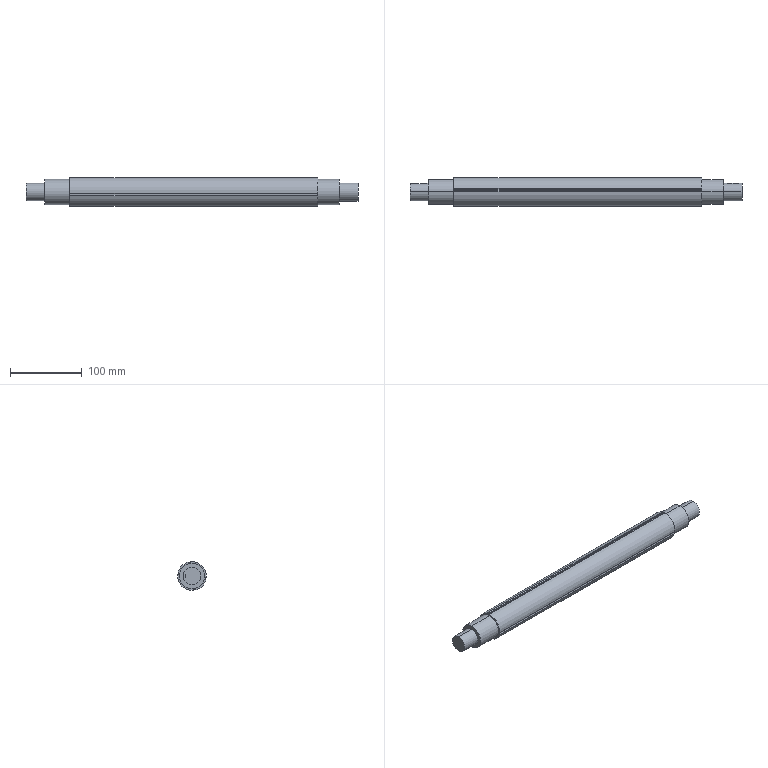Part | SolidWorks | features ICE 7, RefAxis 3, 3DProfileFeature 1, LockFeature 1, MirrorPattern 1, MoveFace 1, Revolution 1 | 1 solid | 34 faces | box 462 x 40 x 40 mm | volume 516055 mm3 | cylinder 22 | plane 12 | commonest cylinder face diameters 4.38 x5 40 x5 8 x4 35 x4 24 x2 25 x2
STEP:
#1=CARTESIAN_POINT('',(185.5,11.843,-4.));
#2=VERTEX_POINT('',#1);
#3=CARTESIAN_POINT('',(185.5,11.843,4.));
#4=VERTEX_POINT('',#3);
#5=CARTESIAN_POINT('',(185.5,11.843,-4.));
#6=CARTESIAN_POINT('',(185.234,11.843,-4.));
#7=CARTESIAN_POINT('',(184.973,11.852,-3.974));
#8=CARTESIAN_POINT('',(184.459,11.886,-3.871));
#9=CARTESIAN_POINT('',(184.204,11.911,-3.793));
#10=CARTESIAN_POINT('',(183.721,11.973,-3.592));
#11=CARTESIAN_POINT('',(183.492,12.01,-3.469));
#12=CARTESIAN_POINT('',(183.059,12.09,-3.179));
#13=CARTESIAN_POINT('',(182.855,12.133,-3.012));
#14=CARTESIAN_POINT('',(182.489,12.218,-2.646));
#15=CARTESIAN_POINT('',(182.324,12.26,-2.445));
#16=CARTESIAN_POINT('',(182.031,12.34,-2.009));
#17=CARTESIAN_POINT('',(181.908,12.375,-1.779));
#18=CARTESIAN_POINT('',(181.708,12.435,-1.299));
#19=CARTESIAN_POINT('',(181.63,12.459,-1.045));
#20=CARTESIAN_POINT('',(181.526,12.492,-0.5276));
#21=CARTESIAN_POINT('',(181.5,12.5,-0.2669));
#22=CARTESIAN_POINT('',(181.5,12.5,0.2587));
#23=CARTESIAN_POINT('',(181.526,12.492,0.5256));
#24=CARTESIAN_POINT('',(181.629,12.459,1.04));
#25=CARTESIAN_POINT('',(181.705,12.436,1.29));
#26=CARTESIAN_POINT('',(181.907,12.375,1.777));
#27=CARTESIAN_POINT('',(182.031,12.34,2.008));
#28=CARTESIAN_POINT('',(182.32,12.262,2.44));
#29=CARTESIAN_POINT('',(182.487,12.219,2.643));
#30=CARTESIAN_POINT('',(182.855,12.133,3.012));
#31=CARTESIAN_POINT('',(183.055,12.091,3.176));
#32=CARTESIAN_POINT('',(183.487,12.011,3.466));
#33=CARTESIAN_POINT('',(183.72,11.973,3.592));
#34=CARTESIAN_POINT('',(184.202,11.911,3.792));
#35=CARTESIAN_POINT('',(184.451,11.886,3.869));
#36=CARTESIAN_POINT('',(184.968,11.852,3.973));
#37=CARTESIAN_POINT('',(185.234,11.843,4.));
#38=CARTESIAN_POINT('',(185.5,11.843,4.));
#39=B_SPLINE_CURVE_WITH_KNOTS('',3,(#5,#6,#7,#8,#9,#10,#11,#12,#13,#14,#15,#16,#17,#18,#19,#20,#21,#22,#23,#24,#25,#26,#27,#28,#29,#30,#31,#32,#33,#34,#35,#36,#37,#38),.UNSPECIFIED.,.F.,.F.,(4,2,2,2,2,2,2,2,2,2,2,2,2,2,2,2,4),(0.,0.0007865,0.001573,0.00236,0.003146,0.003933,0.004719,0.005506,0.006292,0.007079,0.007865,0.008652,0.009438,0.01022,0.01101,0.0118,0.01258),.UNSPECIFIED.);
#40=EDGE_CURVE('',#2,#4,#39,.T.);
#41=ORIENTED_EDGE('',*,*,#40,.F.);
#42=CARTESIAN_POINT('',(200.5,11.843,-4.));
#43=VERTEX_POINT('',#42);
#44=CARTESIAN_POINT('',(179.5,11.843,-4.));
#45=DIRECTION('',(-1.,0.,0.));
#46=VECTOR('',#45,1000.);
#47=LINE('',#44,#46);
#48=EDGE_CURVE('',#43,#2,#47,.T.);
#49=ORIENTED_EDGE('',*,*,#48,.F.);
#50=CARTESIAN_POINT('',(200.5,11.843,4.));
#51=VERTEX_POINT('',#50);
#52=CARTESIAN_POINT('',(200.5,11.843,4.));
#53=CARTESIAN_POINT('',(200.766,11.843,4.));
#54=CARTESIAN_POINT('',(201.027,11.852,3.974));
#55=CARTESIAN_POINT('',(201.541,11.886,3.871));
#56=CARTESIAN_POINT('',(201.796,11.911,3.793));
#57=CARTESIAN_POINT('',(202.279,11.973,3.592));
#58=CARTESIAN_POINT('',(202.508,12.01,3.469));
#59=CARTESIAN_POINT('',(202.941,12.09,3.179));
#60=CARTESIAN_POINT('',(203.145,12.133,3.012));
#61=CARTESIAN_POINT('',(203.511,12.218,2.646));
#62=CARTESIAN_POINT('',(203.676,12.26,2.445));
#63=CARTESIAN_POINT('',(203.969,12.34,2.009));
#64=CARTESIAN_POINT('',(204.092,12.375,1.779));
#65=CARTESIAN_POINT('',(204.292,12.435,1.299));
#66=CARTESIAN_POINT('',(204.37,12.459,1.045));
#67=CARTESIAN_POINT('',(204.474,12.492,0.5276));
#68=CARTESIAN_POINT('',(204.5,12.5,0.2669));
#69=CARTESIAN_POINT('',(204.5,12.5,-0.2587));
#70=CARTESIAN_POINT('',(204.474,12.492,-0.5256));
#71=CARTESIAN_POINT('',(204.371,12.459,-1.04));
#72=CARTESIAN_POINT('',(204.295,12.436,-1.29));
#73=CARTESIAN_POINT('',(204.093,12.375,-1.777));
#74=CARTESIAN_POINT('',(203.969,12.34,-2.008));
#75=CARTESIAN_POINT('',(203.68,12.262,-2.44));
#76=CARTESIAN_POINT('',(203.513,12.219,-2.643));
#77=CARTESIAN_POINT('',(203.145,12.133,-3.012));
#78=CARTESIAN_POINT('',(202.945,12.091,-3.176));
#79=CARTESIAN_POINT('',(202.513,12.011,-3.466));
#80=CARTESIAN_POINT('',(202.28,11.973,-3.592));
#81=CARTESIAN_POINT('',(201.798,11.911,-3.792));
#82=CARTESIAN_POINT('',(201.549,11.886,-3.869));
#83=CARTESIAN_POINT('',(201.032,11.852,-3.973));
#84=CARTESIAN_POINT('',(200.766,11.843,-4.));
#85=CARTESIAN_POINT('',(200.5,11.843,-4.));
#86=B_SPLINE_CURVE_WITH_KNOTS('',3,(#52,#53,#54,#55,#56,#57,#58,#59,#60,#61,#62,#63,#64,#65,#66,#67,#68,#69,#70,#71,#72,#73,#74,#75,#76,#77,#78,#79,#80,#81,#82,#83,#84,#85),.UNSPECIFIED.,.F.,.F.,(4,2,2,2,2,2,2,2,2,2,2,2,2,2,2,2,4),(0.,0.0007865,0.001573,0.00236,0.003146,0.003933,0.004719,0.005506,0.006292,0.007079,0.007865,0.008652,0.009438,0.01022,0.01101,0.0118,0.01258),.UNSPECIFIED.);
#87=EDGE_CURVE('',#51,#43,#86,.T.);
#88=ORIENTED_EDGE('',*,*,#87,.F.);
#89=CARTESIAN_POINT('',(179.5,11.843,4.));
#90=DIRECTION('',(1.,0.,0.));
#91=VECTOR('',#90,1000.);
#92=LINE('',#89,#91);
#93=EDGE_CURVE('',#4,#51,#92,.T.);
#94=ORIENTED_EDGE('',*,*,#93,.F.);
#95=EDGE_LOOP('',(#41,#49,#88,#94));
#96=FACE_BOUND('',#95,.T.);
#97=CARTESIAN_POINT('',(179.5,0.,-12.5));
#98=VERTEX_POINT('',#97);
#99=CARTESIAN_POINT('',(179.5,0.,12.5));
#100=VERTEX_POINT('',#99);
#101=CARTESIAN_POINT('',(179.5,0.,0.));
#102=DIRECTION('',(1.,0.,0.));
#103=DIRECTION('',(0.,0.,-1.));
#104=AXIS2_PLACEMENT_3D('',#101,#102,#103);
#105=CIRCLE('',#104,12.5);
#106=EDGE_CURVE('',#98,#100,#105,.T.);
#107=ORIENTED_EDGE('',*,*,#106,.T.);
#108=CARTESIAN_POINT('',(205.5,0.,12.5));
#109=VERTEX_POINT('',#108);
#110=CARTESIAN_POINT('',(179.5,0.,12.5));
#111=DIRECTION('',(1.,0.,0.));
#112=VECTOR('',#111,1000.);
#113=LINE('',#110,#112);
#114=EDGE_CURVE('',#100,#109,#113,.T.);
#115=ORIENTED_EDGE('',*,*,#114,.T.);
#116=CARTESIAN_POINT('',(205.5,0.,-12.5));
#117=VERTEX_POINT('',#116);
#118=CARTESIAN_POINT('',(205.5,0.,0.));
#119=DIRECTION('',(1.,0.,0.));
#120=DIRECTION('',(0.,0.,-1.));
#121=AXIS2_PLACEMENT_3D('',#118,#119,#120);
#122=CIRCLE('',#121,12.5);
#123=EDGE_CURVE('',#117,#109,#122,.T.);
#124=ORIENTED_EDGE('',*,*,#123,.F.);
#125=CARTESIAN_POINT('',(179.5,0.,-12.5));
#126=DIRECTION('',(1.,0.,0.));
#127=VECTOR('',#126,1000.);
#128=LINE('',#125,#127);
#129=EDGE_CURVE('',#98,#117,#128,.T.);
#130=ORIENTED_EDGE('',*,*,#129,.F.);
#131=EDGE_LOOP('',(#107,#115,#124,#130));
#132=FACE_OUTER_BOUND('',#131,.T.);
#133=CARTESIAN_POINT('',(179.5,0.,0.));
#134=DIRECTION('',(1.,0.,0.));
#135=DIRECTION('',(0.,0.,-1.));
#136=AXIS2_PLACEMENT_3D('',#133,#134,#135);
#137=CYLINDRICAL_SURFACE('',#136,12.5);
#138=ADVANCED_FACE('',(#96,#132),#137,.T.);
#139=CARTESIAN_POINT('',(149.5,0.,-17.5));
#140=VERTEX_POINT('',#139);
#141=CARTESIAN_POINT('',(149.5,0.,17.5));
#142=VERTEX_POINT('',#141);
#143=CARTESIAN_POINT('',(149.5,0.,0.));
#144=DIRECTION('',(1.,0.,0.));
#145=DIRECTION('',(0.,0.,-1.));
#146=AXIS2_PLACEMENT_3D('',#143,#144,#145);
#147=CIRCLE('',#146,17.5);
#148=EDGE_CURVE('',#140,#142,#147,.T.);
#149=ORIENTED_EDGE('',*,*,#148,.T.);
#150=CARTESIAN_POINT('',(179.5,0.,17.5));
#151=VERTEX_POINT('',#150);
#152=CARTESIAN_POINT('',(149.5,0.,17.5));
#153=DIRECTION('',(1.,0.,0.));
#154=VECTOR('',#153,1000.);
#155=LINE('',#152,#154);
#156=EDGE_CURVE('',#142,#151,#155,.T.);
#157=ORIENTED_EDGE('',*,*,#156,.T.);
#158=CARTESIAN_POINT('',(179.5,0.,-17.5));
#159=VERTEX_POINT('',#158);
#160=CARTESIAN_POINT('',(179.5,0.,0.));
#161=DIRECTION('',(1.,0.,0.));
#162=DIRECTION('',(0.,0.,-1.));
#163=AXIS2_PLACEMENT_3D('',#160,#161,#162);
#164=CIRCLE('',#163,17.5);
#165=EDGE_CURVE('',#159,#151,#164,.T.);
#166=ORIENTED_EDGE('',*,*,#165,.F.);
#167=CARTESIAN_POINT('',(149.5,0.,-17.5));
#168=DIRECTION('',(1.,0.,0.));
#169=VECTOR('',#168,1000.);
#170=LINE('',#167,#169);
#171=EDGE_CURVE('',#140,#159,#170,.T.);
#172=ORIENTED_EDGE('',*,*,#171,.F.);
#173=EDGE_LOOP('',(#149,#157,#166,#172));
#174=FACE_OUTER_BOUND('',#173,.T.);
#175=CARTESIAN_POINT('',(149.5,0.,0.));
#176=DIRECTION('',(1.,0.,0.));
#177=DIRECTION('',(0.,0.,-1.));
#178=AXIS2_PLACEMENT_3D('',#175,#176,#177);
#179=CYLINDRICAL_SURFACE('',#178,17.5);
#180=ADVANCED_FACE('',(#174),#179,.T.);
#181=CARTESIAN_POINT('',(-195.5,5.203,19.311));
#182=VERTEX_POINT('',#181);
#183=CARTESIAN_POINT('',(-195.5,3.683,18.698));
#184=VERTEX_POINT('',#183);
#185=CARTESIAN_POINT('',(-195.5,3.683,20.888));
#186=DIRECTION('',(-1.,0.,0.));
#187=DIRECTION('',(0.,0.,1.));
#188=AXIS2_PLACEMENT_3D('',#185,#186,#187);
#189=CIRCLE('',#188,2.19);
#190=EDGE_CURVE('',#182,#184,#189,.T.);
#191=ORIENTED_EDGE('',*,*,#190,.T.);
#192=CARTESIAN_POINT('',(149.5,3.683,18.698));
#193=VERTEX_POINT('',#192);
#194=CARTESIAN_POINT('',(-205.5,3.683,18.698));
#195=DIRECTION('',(1.,0.,0.));
#196=VECTOR('',#195,1000.);
#197=LINE('',#194,#196);
#198=EDGE_CURVE('',#184,#193,#197,.T.);
#199=ORIENTED_EDGE('',*,*,#198,.T.);
#200=CARTESIAN_POINT('',(149.5,5.203,19.311));
#201=VERTEX_POINT('',#200);
#202=CARTESIAN_POINT('',(149.5,3.683,20.888));
#203=DIRECTION('',(1.,0.,0.));
#204=DIRECTION('',(0.,0.,-1.));
#205=AXIS2_PLACEMENT_3D('',#202,#203,#204);
#206=CIRCLE('',#205,2.19);
#207=EDGE_CURVE('',#193,#201,#206,.T.);
#208=ORIENTED_EDGE('',*,*,#207,.T.);
#209=CARTESIAN_POINT('',(-205.5,5.203,19.311));
#210=DIRECTION('',(1.,0.,0.));
#211=VECTOR('',#210,1000.);
#212=LINE('',#209,#211);
#213=EDGE_CURVE('',#182,#201,#212,.T.);
#214=ORIENTED_EDGE('',*,*,#213,.F.);
#215=EDGE_LOOP('',(#191,#199,#208,#214));
#216=FACE_OUTER_BOUND('',#215,.T.);
#217=CARTESIAN_POINT('',(-205.5,3.683,20.888));
#218=DIRECTION('',(1.,0.,0.));
#219=DIRECTION('',(0.,0.,-1.));
#220=AXIS2_PLACEMENT_3D('',#217,#218,#219);
#221=CYLINDRICAL_SURFACE('',#220,2.19);
#222=ADVANCED_FACE('',(#216),#221,.F.);
#223=CARTESIAN_POINT('',(149.5,0.,20.));
#224=VERTEX_POINT('',#223);
#225=CARTESIAN_POINT('',(149.5,-19.926,-1.715));
#226=VERTEX_POINT('',#225);
#227=CARTESIAN_POINT('',(149.5,0.,0.));
#228=DIRECTION('',(1.,0.,0.));
#229=DIRECTION('',(0.,0.,-1.));
#230=AXIS2_PLACEMENT_3D('',#227,#228,#229);
#231=CIRCLE('',#230,20.);
#232=EDGE_CURVE('',#224,#226,#231,.T.);
#233=ORIENTED_EDGE('',*,*,#232,.F.);
#234=CARTESIAN_POINT('',(-195.5,0.,20.));
#235=VERTEX_POINT('',#234);
#236=CARTESIAN_POINT('',(205.5,0.,20.));
#237=DIRECTION('',(-1.,0.,0.));
#238=VECTOR('',#237,1000.);
#239=LINE('',#236,#238);
#240=EDGE_CURVE('',#224,#235,#239,.T.);
#241=ORIENTED_EDGE('',*,*,#240,.T.);
#242=CARTESIAN_POINT('',(-195.5,-19.926,-1.715));
#243=VERTEX_POINT('',#242);
#244=CARTESIAN_POINT('',(-195.5,0.,0.));
#245=DIRECTION('',(-1.,0.,0.));
#246=DIRECTION('',(0.,0.,1.));
#247=AXIS2_PLACEMENT_3D('',#244,#245,#246);
#248=CIRCLE('',#247,20.);
#249=EDGE_CURVE('',#243,#235,#248,.T.);
#250=ORIENTED_EDGE('',*,*,#249,.F.);
#251=CARTESIAN_POINT('',(-205.5,-19.926,-1.715));
#252=DIRECTION('',(1.,0.,0.));
#253=VECTOR('',#252,1000.);
#254=LINE('',#251,#253);
#255=EDGE_CURVE('',#243,#226,#254,.T.);
#256=ORIENTED_EDGE('',*,*,#255,.T.);
#257=EDGE_LOOP('',(#233,#241,#250,#256));
#258=FACE_OUTER_BOUND('',#257,.T.);
#259=CARTESIAN_POINT('',(205.5,0.,0.));
#260=DIRECTION('',(-1.,0.,0.));
#261=DIRECTION('',(0.,0.,1.));
#262=AXIS2_PLACEMENT_3D('',#259,#260,#261);
#263=CYLINDRICAL_SURFACE('',#262,20.);
#264=ADVANCED_FACE('',(#258),#263,.T.);
#265=CARTESIAN_POINT('',(-195.5,0.,17.5));
#266=VERTEX_POINT('',#265);
#267=CARTESIAN_POINT('',(-195.5,0.,-17.5));
#268=VERTEX_POINT('',#267);
#269=CARTESIAN_POINT('',(-195.5,0.,0.));
#270=DIRECTION('',(-1.,0.,0.));
#271=DIRECTION('',(0.,0.,1.));
#272=AXIS2_PLACEMENT_3D('',#269,#270,#271);
#273=CIRCLE('',#272,17.5);
#274=EDGE_CURVE('',#266,#268,#273,.T.);
#275=ORIENTED_EDGE('',*,*,#274,.T.);
#276=CARTESIAN_POINT('',(-230.5,0.,-17.5));
#277=VERTEX_POINT('',#276);
#278=CARTESIAN_POINT('',(-187.5,0.,-17.5));
#279=DIRECTION('',(-1.,0.,0.));
#280=VECTOR('',#279,1000.);
#281=LINE('',#278,#280);
#282=EDGE_CURVE('',#268,#277,#281,.T.);
#283=ORIENTED_EDGE('',*,*,#282,.T.);
#284=CARTESIAN_POINT('',(-230.5,0.,17.5));
#285=VERTEX_POINT('',#284);
#286=CARTESIAN_POINT('',(-230.5,0.,0.));
#287=DIRECTION('',(1.,0.,0.));
#288=DIRECTION('',(0.,0.,1.));
#289=AXIS2_PLACEMENT_3D('',#286,#287,#288);
#290=CIRCLE('',#289,17.5);
#291=EDGE_CURVE('',#277,#285,#290,.T.);
#292=ORIENTED_EDGE('',*,*,#291,.T.);
#293=CARTESIAN_POINT('',(-187.5,0.,17.5));
#294=DIRECTION('',(-1.,0.,0.));
#295=VECTOR('',#294,1000.);
#296=LINE('',#293,#295);
#297=EDGE_CURVE('',#266,#285,#296,.T.);
#298=ORIENTED_EDGE('',*,*,#297,.F.);
#299=EDGE_LOOP('',(#275,#283,#292,#298));
#300=FACE_OUTER_BOUND('',#299,.T.);
#301=CARTESIAN_POINT('',(-187.5,0.,0.));
#302=DIRECTION('',(-1.,0.,0.));
#303=DIRECTION('',(0.,0.,1.));
#304=AXIS2_PLACEMENT_3D('',#301,#302,#303);
#305=CYLINDRICAL_SURFACE('',#304,17.5);
#306=ADVANCED_FACE('',(#300),#305,.T.);
#307=CARTESIAN_POINT('',(-236.5,11.314,4.));
#308=VERTEX_POINT('',#307);
#309=CARTESIAN_POINT('',(-251.5,11.314,4.));
#310=VERTEX_POINT('',#309);
#311=CARTESIAN_POINT('',(-230.5,11.314,4.));
#312=DIRECTION('',(-1.,0.,0.));
#313=VECTOR('',#312,1000.);
#314=LINE('',#311,#313);
#315=EDGE_CURVE('',#308,#310,#314,.T.);
#316=ORIENTED_EDGE('',*,*,#315,.T.);
#317=CARTESIAN_POINT('',(-251.5,11.314,-4.));
#318=VERTEX_POINT('',#317);
#319=CARTESIAN_POINT('',(-251.5,11.314,4.));
#320=CARTESIAN_POINT('',(-251.766,11.314,4.));
#321=CARTESIAN_POINT('',(-252.028,11.323,3.974));
#322=CARTESIAN_POINT('',(-252.541,11.359,3.871));
#323=CARTESIAN_POINT('',(-252.796,11.385,3.793));
#324=CARTESIAN_POINT('',(-253.279,11.45,3.592));
#325=CARTESIAN_POINT('',(-253.508,11.489,3.469));
#326=CARTESIAN_POINT('',(-253.942,11.572,3.179));
#327=CARTESIAN_POINT('',(-254.145,11.617,3.012));
#328=CARTESIAN_POINT('',(-254.511,11.706,2.646));
#329=CARTESIAN_POINT('',(-254.676,11.75,2.446));
#330=CARTESIAN_POINT('',(-254.969,11.833,2.009));
#331=CARTESIAN_POINT('',(-255.092,11.87,1.78));
#332=CARTESIAN_POINT('',(-255.292,11.932,1.299));
#333=CARTESIAN_POINT('',(-255.37,11.957,1.045));
#334=CARTESIAN_POINT('',(-255.474,11.991,0.528));
#335=CARTESIAN_POINT('',(-255.5,12.,0.2672));
#336=CARTESIAN_POINT('',(-255.5,12.,-0.2587));
#337=CARTESIAN_POINT('',(-255.474,11.991,-0.5259));
#338=CARTESIAN_POINT('',(-255.371,11.958,-1.04));
#339=CARTESIAN_POINT('',(-255.295,11.933,-1.291));
#340=CARTESIAN_POINT('',(-255.093,11.87,-1.778));
#341=CARTESIAN_POINT('',(-254.969,11.833,-2.009));
#342=CARTESIAN_POINT('',(-254.68,11.751,-2.44));
#343=CARTESIAN_POINT('',(-254.513,11.707,-2.644));
#344=CARTESIAN_POINT('',(-254.145,11.617,-3.012));
#345=CARTESIAN_POINT('',(-253.945,11.573,-3.176));
#346=CARTESIAN_POINT('',(-253.514,11.49,-3.466));
#347=CARTESIAN_POINT('',(-253.28,11.45,-3.592));
#348=CARTESIAN_POINT('',(-252.799,11.386,-3.792));
#349=CARTESIAN_POINT('',(-252.55,11.359,-3.869));
#350=CARTESIAN_POINT('',(-252.032,11.323,-3.973));
#351=CARTESIAN_POINT('',(-251.766,11.314,-4.));
#352=CARTESIAN_POINT('',(-251.5,11.314,-4.));
#353=B_SPLINE_CURVE_WITH_KNOTS('',3,(#319,#320,#321,#322,#323,#324,#325,#326,#327,#328,#329,#330,#331,#332,#333,#334,#335,#336,#337,#338,#339,#340,#341,#342,#343,#344,#345,#346,#347,#348,#349,#350,#351,#352),.UNSPECIFIED.,.F.,.F.,(4,2,2,2,2,2,2,2,2,2,2,2,2,2,2,2,4),(0.,0.000787,0.001574,0.002361,0.003148,0.003935,0.004722,0.005509,0.006296,0.007083,0.00787,0.008657,0.009444,0.01023,0.01102,0.0118,0.01259),.UNSPECIFIED.);
#354=EDGE_CURVE('',#310,#318,#353,.T.);
#355=ORIENTED_EDGE('',*,*,#354,.T.);
#356=CARTESIAN_POINT('',(-236.5,11.314,-4.));
#357=VERTEX_POINT('',#356);
#358=CARTESIAN_POINT('',(-230.5,11.314,-4.));
#359=DIRECTION('',(1.,0.,0.));
#360=VECTOR('',#359,1000.);
#361=LINE('',#358,#360);
#362=EDGE_CURVE('',#318,#357,#361,.T.);
#363=ORIENTED_EDGE('',*,*,#362,.T.);
#364=CARTESIAN_POINT('',(-236.5,11.314,-4.));
#365=CARTESIAN_POINT('',(-236.234,11.314,-4.));
#366=CARTESIAN_POINT('',(-235.972,11.323,-3.974));
#367=CARTESIAN_POINT('',(-235.459,11.359,-3.871));
#368=CARTESIAN_POINT('',(-235.204,11.385,-3.793));
#369=CARTESIAN_POINT('',(-234.721,11.45,-3.592));
#370=CARTESIAN_POINT('',(-234.492,11.489,-3.469));
#371=CARTESIAN_POINT('',(-234.058,11.572,-3.179));
#372=CARTESIAN_POINT('',(-233.855,11.617,-3.012));
#373=CARTESIAN_POINT('',(-233.489,11.706,-2.646));
#374=CARTESIAN_POINT('',(-233.324,11.75,-2.446));
#375=CARTESIAN_POINT('',(-233.031,11.833,-2.009));
#376=CARTESIAN_POINT('',(-232.908,11.87,-1.78));
#377=CARTESIAN_POINT('',(-232.708,11.932,-1.299));
#378=CARTESIAN_POINT('',(-232.63,11.957,-1.045));
#379=CARTESIAN_POINT('',(-232.526,11.991,-0.528));
#380=CARTESIAN_POINT('',(-232.5,12.,-0.2672));
#381=CARTESIAN_POINT('',(-232.5,12.,0.2587));
#382=CARTESIAN_POINT('',(-232.526,11.991,0.5259));
#383=CARTESIAN_POINT('',(-232.629,11.958,1.04));
#384=CARTESIAN_POINT('',(-232.705,11.933,1.291));
#385=CARTESIAN_POINT('',(-232.907,11.87,1.778));
#386=CARTESIAN_POINT('',(-233.031,11.833,2.009));
#387=CARTESIAN_POINT('',(-233.32,11.751,2.44));
#388=CARTESIAN_POINT('',(-233.487,11.707,2.644));
#389=CARTESIAN_POINT('',(-233.855,11.617,3.012));
#390=CARTESIAN_POINT('',(-234.055,11.573,3.176));
#391=CARTESIAN_POINT('',(-234.486,11.49,3.466));
#392=CARTESIAN_POINT('',(-234.72,11.45,3.592));
#393=CARTESIAN_POINT('',(-235.201,11.386,3.792));
#394=CARTESIAN_POINT('',(-235.45,11.359,3.869));
#395=CARTESIAN_POINT('',(-235.968,11.323,3.973));
#396=CARTESIAN_POINT('',(-236.234,11.314,4.));
#397=CARTESIAN_POINT('',(-236.5,11.314,4.));
#398=B_SPLINE_CURVE_WITH_KNOTS('',3,(#364,#365,#366,#367,#368,#369,#370,#371,#372,#373,#374,#375,#376,#377,#378,#379,#380,#381,#382,#383,#384,#385,#386,#387,#388,#389,#390,#391,#392,#393,#394,#395,#396,#397),.UNSPECIFIED.,.F.,.F.,(4,2,2,2,2,2,2,2,2,2,2,2,2,2,2,2,4),(0.,0.000787,0.001574,0.002361,0.003148,0.003935,0.004722,0.005509,0.006296,0.007083,0.00787,0.008657,0.009444,0.01023,0.01102,0.0118,0.01259),.UNSPECIFIED.);
#399=EDGE_CURVE('',#357,#308,#398,.T.);
#400=ORIENTED_EDGE('',*,*,#399,.T.);
#401=EDGE_LOOP('',(#316,#355,#363,#400));
#402=FACE_BOUND('',#401,.T.);
#403=CARTESIAN_POINT('',(-230.5,0.,12.));
#404=VERTEX_POINT('',#403);
#405=CARTESIAN_POINT('',(-230.5,0.,-12.));
#406=VERTEX_POINT('',#405);
#407=CARTESIAN_POINT('',(-230.5,0.,0.));
#408=DIRECTION('',(-1.,0.,0.));
#409=DIRECTION('',(0.,0.,1.));
#410=AXIS2_PLACEMENT_3D('',#407,#408,#409);
#411=CIRCLE('',#410,12.);
#412=EDGE_CURVE('',#404,#406,#411,.T.);
#413=ORIENTED_EDGE('',*,*,#412,.T.);
#414=CARTESIAN_POINT('',(-256.5,0.,-12.));
#415=VERTEX_POINT('',#414);
#416=CARTESIAN_POINT('',(-230.5,0.,-12.));
#417=DIRECTION('',(-1.,0.,0.));
#418=VECTOR('',#417,1000.);
#419=LINE('',#416,#418);
#420=EDGE_CURVE('',#406,#415,#419,.T.);
#421=ORIENTED_EDGE('',*,*,#420,.T.);
#422=CARTESIAN_POINT('',(-256.5,0.,12.));
#423=VERTEX_POINT('',#422);
#424=CARTESIAN_POINT('',(-256.5,0.,0.));
#425=DIRECTION('',(-1.,0.,0.));
#426=DIRECTION('',(0.,0.,1.));
#427=AXIS2_PLACEMENT_3D('',#424,#425,#426);
#428=CIRCLE('',#427,12.);
#429=EDGE_CURVE('',#423,#415,#428,.T.);
#430=ORIENTED_EDGE('',*,*,#429,.F.);
#431=CARTESIAN_POINT('',(-230.5,0.,12.));
#432=DIRECTION('',(-1.,0.,0.));
#433=VECTOR('',#432,1000.);
#434=LINE('',#431,#433);
#435=EDGE_CURVE('',#404,#423,#434,.T.);
#436=ORIENTED_EDGE('',*,*,#435,.F.);
#437=EDGE_LOOP('',(#413,#421,#430,#436));
#438=FACE_OUTER_BOUND('',#437,.T.);
#439=CARTESIAN_POINT('',(-230.5,0.,0.));
#440=DIRECTION('',(-1.,0.,0.));
#441=DIRECTION('',(0.,0.,1.));
#442=AXIS2_PLACEMENT_3D('',#439,#440,#441);
#443=CYLINDRICAL_SURFACE('',#442,12.);
#444=ADVANCED_FACE('',(#402,#438),#443,.T.);
#445=ORIENTED_EDGE('',*,*,#420,.F.);
#446=CARTESIAN_POINT('',(-230.5,0.,0.));
#447=DIRECTION('',(-1.,0.,0.));
#448=DIRECTION('',(0.,0.,1.));
#449=AXIS2_PLACEMENT_3D('',#446,#447,#448);
#450=CIRCLE('',#449,12.);
#451=EDGE_CURVE('',#406,#404,#450,.T.);
#452=ORIENTED_EDGE('',*,*,#451,.T.);
#453=ORIENTED_EDGE('',*,*,#435,.T.);
#454=CARTESIAN_POINT('',(-256.5,0.,0.));
#455=DIRECTION('',(-1.,0.,0.));
#456=DIRECTION('',(0.,0.,1.));
#457=AXIS2_PLACEMENT_3D('',#454,#455,#456);
#458=CIRCLE('',#457,12.);
#459=EDGE_CURVE('',#415,#423,#458,.T.);
#460=ORIENTED_EDGE('',*,*,#459,.F.);
#461=EDGE_LOOP('',(#445,#452,#453,#460));
#462=FACE_OUTER_BOUND('',#461,.T.);
#463=CARTESIAN_POINT('',(-230.5,0.,0.));
#464=DIRECTION('',(-1.,0.,0.));
#465=DIRECTION('',(0.,0.,1.));
#466=AXIS2_PLACEMENT_3D('',#463,#464,#465);
#467=CYLINDRICAL_SURFACE('',#466,12.);
#468=ADVANCED_FACE('',(#462),#467,.T.);
#469=ORIENTED_EDGE('',*,*,#282,.F.);
#470=CARTESIAN_POINT('',(-195.5,0.,0.));
#471=DIRECTION('',(-1.,0.,0.));
#472=DIRECTION('',(0.,0.,1.));
#473=AXIS2_PLACEMENT_3D('',#470,#471,#472);
#474=CIRCLE('',#473,17.5);
#475=EDGE_CURVE('',#268,#266,#474,.T.);
#476=ORIENTED_EDGE('',*,*,#475,.T.);
#477=ORIENTED_EDGE('',*,*,#297,.T.);
#478=CARTESIAN_POINT('',(-230.5,0.,0.));
#479=DIRECTION('',(1.,0.,0.));
#480=DIRECTION('',(0.,0.,1.));
#481=AXIS2_PLACEMENT_3D('',#478,#479,#480);
#482=CIRCLE('',#481,17.5);
#483=EDGE_CURVE('',#285,#277,#482,.T.);
#484=ORIENTED_EDGE('',*,*,#483,.T.);
#485=EDGE_LOOP('',(#469,#476,#477,#484));
#486=FACE_OUTER_BOUND('',#485,.T.);
#487=CARTESIAN_POINT('',(-187.5,0.,0.));
#488=DIRECTION('',(-1.,0.,0.));
#489=DIRECTION('',(0.,0.,1.));
#490=AXIS2_PLACEMENT_3D('',#487,#488,#489);
#491=CYLINDRICAL_SURFACE('',#490,17.5);
#492=ADVANCED_FACE('',(#486),#491,.T.);
#493=CARTESIAN_POINT('',(149.5,19.311,5.203));
#494=VERTEX_POINT('',#493);
#495=CARTESIAN_POINT('',(149.5,0.,0.));
#496=DIRECTION('',(1.,0.,0.));
#497=DIRECTION('',(0.,0.,-1.));
#498=AXIS2_PLACEMENT_3D('',#495,#496,#497);
#499=CIRCLE('',#498,20.);
#500=EDGE_CURVE('',#494,#201,#499,.T.);
#501=ORIENTED_EDGE('',*,*,#500,.F.);
#502=CARTESIAN_POINT('',(-195.5,19.311,5.203));
#503=VERTEX_POINT('',#502);
#504=CARTESIAN_POINT('',(-205.5,19.311,5.203));
#505=DIRECTION('',(1.,0.,0.));
#506=VECTOR('',#505,1000.);
#507=LINE('',#504,#506);
#508=EDGE_CURVE('',#503,#494,#507,.T.);
#509=ORIENTED_EDGE('',*,*,#508,.F.);
#510=CARTESIAN_POINT('',(-195.5,0.,0.));
#511=DIRECTION('',(-1.,0.,0.));
#512=DIRECTION('',(0.,0.,1.));
#513=AXIS2_PLACEMENT_3D('',#510,#511,#512);
#514=CIRCLE('',#513,20.);
#515=EDGE_CURVE('',#182,#503,#514,.T.);
#516=ORIENTED_EDGE('',*,*,#515,.F.);
#517=ORIENTED_EDGE('',*,*,#213,.T.);
#518=EDGE_LOOP('',(#501,#509,#516,#517));
#519=FACE_OUTER_BOUND('',#518,.T.);
#520=CARTESIAN_POINT('',(205.5,0.,0.));
#521=DIRECTION('',(-1.,0.,0.));
#522=DIRECTION('',(0.,0.,1.));
#523=AXIS2_PLACEMENT_3D('',#520,#521,#522);
#524=CYLINDRICAL_SURFACE('',#523,20.);
#525=ADVANCED_FACE('',(#519),#524,.T.);
#526=ORIENTED_EDGE('',*,*,#240,.F.);
#527=CARTESIAN_POINT('',(149.5,1.715,19.926));
#528=VERTEX_POINT('',#527);
#529=CARTESIAN_POINT('',(149.5,0.,0.));
#530=DIRECTION('',(1.,0.,0.));
#531=DIRECTION('',(0.,0.,-1.));
#532=AXIS2_PLACEMENT_3D('',#529,#530,#531);
#533=CIRCLE('',#532,20.);
#534=EDGE_CURVE('',#528,#224,#533,.T.);
#535=ORIENTED_EDGE('',*,*,#534,.F.);
#536=CARTESIAN_POINT('',(-195.5,1.715,19.926));
#537=VERTEX_POINT('',#536);
#538=CARTESIAN_POINT('',(-205.5,1.715,19.926));
#539=DIRECTION('',(1.,0.,0.));
#540=VECTOR('',#539,1000.);
#541=LINE('',#538,#540);
#542=EDGE_CURVE('',#537,#528,#541,.T.);
#543=ORIENTED_EDGE('',*,*,#542,.F.);
#544=CARTESIAN_POINT('',(-195.5,0.,0.));
#545=DIRECTION('',(-1.,0.,0.));
#546=DIRECTION('',(0.,0.,1.));
#547=AXIS2_PLACEMENT_3D('',#544,#545,#546);
#548=CIRCLE('',#547,20.);
#549=EDGE_CURVE('',#235,#537,#548,.T.);
#550=ORIENTED_EDGE('',*,*,#549,.F.);
#551=EDGE_LOOP('',(#526,#535,#543,#550));
#552=FACE_OUTER_BOUND('',#551,.T.);
#553=CARTESIAN_POINT('',(205.5,0.,0.));
#554=DIRECTION('',(-1.,0.,0.));
#555=DIRECTION('',(0.,0.,1.));
#556=AXIS2_PLACEMENT_3D('',#553,#554,#555);
#557=CYLINDRICAL_SURFACE('',#556,20.);
#558=ADVANCED_FACE('',(#552),#557,.T.);
#559=CARTESIAN_POINT('',(149.5,-1.715,-19.926));
#560=VERTEX_POINT('',#559);
#561=CARTESIAN_POINT('',(149.5,19.926,1.715));
#562=VERTEX_POINT('',#561);
#563=CARTESIAN_POINT('',(149.5,0.,0.));
#564=DIRECTION('',(1.,0.,0.));
#565=DIRECTION('',(0.,0.,-1.));
#566=AXIS2_PLACEMENT_3D('',#563,#564,#565);
#567=CIRCLE('',#566,20.);
#568=EDGE_CURVE('',#560,#562,#567,.T.);
#569=ORIENTED_EDGE('',*,*,#568,.F.);
#570=CARTESIAN_POINT('',(-195.5,-1.715,-19.926));
#571=VERTEX_POINT('',#570);
#572=CARTESIAN_POINT('',(-205.5,-1.715,-19.926));
#573=DIRECTION('',(1.,0.,0.));
#574=VECTOR('',#573,1000.);
#575=LINE('',#572,#574);
#576=EDGE_CURVE('',#571,#560,#575,.T.);
#577=ORIENTED_EDGE('',*,*,#576,.F.);
#578=CARTESIAN_POINT('',(-195.5,19.926,1.715));
#579=VERTEX_POINT('',#578);
#580=CARTESIAN_POINT('',(-195.5,0.,0.));
#581=DIRECTION('',(-1.,0.,0.));
#582=DIRECTION('',(0.,0.,1.));
#583=AXIS2_PLACEMENT_3D('',#580,#581,#582);
#584=CIRCLE('',#583,20.);
#585=EDGE_CURVE('',#579,#571,#584,.T.);
#586=ORIENTED_EDGE('',*,*,#585,.F.);
#587=CARTESIAN_POINT('',(-205.5,19.926,1.715));
#588=DIRECTION('',(1.,0.,0.));
#589=VECTOR('',#588,1000.);
#590=LINE('',#587,#589);
#591=EDGE_CURVE('',#579,#562,#590,.T.);
#592=ORIENTED_EDGE('',*,*,#591,.T.);
#593=EDGE_LOOP('',(#569,#577,#586,#592));
#594=FACE_OUTER_BOUND('',#593,.T.);
#595=CARTESIAN_POINT('',(205.5,0.,0.));
#596=DIRECTION('',(-1.,0.,0.));
#597=DIRECTION('',(0.,0.,1.));
#598=AXIS2_PLACEMENT_3D('',#595,#596,#597);
#599=CYLINDRICAL_SURFACE('',#598,20.);
#600=ADVANCED_FACE('',(#594),#599,.T.);
#601=CARTESIAN_POINT('',(149.5,-19.311,-5.203));
#602=VERTEX_POINT('',#601);
#603=CARTESIAN_POINT('',(149.5,-5.203,-19.311));
#604=VERTEX_POINT('',#603);
#605=CARTESIAN_POINT('',(149.5,0.,0.));
#606=DIRECTION('',(1.,0.,0.));
#607=DIRECTION('',(0.,0.,-1.));
#608=AXIS2_PLACEMENT_3D('',#605,#606,#607);
#609=CIRCLE('',#608,20.);
#610=EDGE_CURVE('',#602,#604,#609,.T.);
#611=ORIENTED_EDGE('',*,*,#610,.F.);
#612=CARTESIAN_POINT('',(-195.5,-19.311,-5.203));
#613=VERTEX_POINT('',#612);
#614=CARTESIAN_POINT('',(-205.5,-19.311,-5.203));
#615=DIRECTION('',(1.,0.,0.));
#616=VECTOR('',#615,1000.);
#617=LINE('',#614,#616);
#618=EDGE_CURVE('',#613,#602,#617,.T.);
#619=ORIENTED_EDGE('',*,*,#618,.F.);
#620=CARTESIAN_POINT('',(-195.5,-5.203,-19.311));
#621=VERTEX_POINT('',#620);
#622=CARTESIAN_POINT('',(-195.5,0.,0.));
#623=DIRECTION('',(-1.,0.,0.));
#624=DIRECTION('',(0.,0.,1.));
#625=AXIS2_PLACEMENT_3D('',#622,#623,#624);
#626=CIRCLE('',#625,20.);
#627=EDGE_CURVE('',#621,#613,#626,.T.);
#628=ORIENTED_EDGE('',*,*,#627,.F.);
#629=CARTESIAN_POINT('',(-205.5,-5.203,-19.311));
#630=DIRECTION('',(1.,0.,0.));
#631=VECTOR('',#630,1000.);
#632=LINE('',#629,#631);
#633=EDGE_CURVE('',#621,#604,#632,.T.);
#634=ORIENTED_EDGE('',*,*,#633,.T.);
#635=EDGE_LOOP('',(#611,#619,#628,#634));
#636=FACE_OUTER_BOUND('',#635,.T.);
#637=CARTESIAN_POINT('',(205.5,0.,0.));
#638=DIRECTION('',(-1.,0.,0.));
#639=DIRECTION('',(0.,0.,1.));
#640=AXIS2_PLACEMENT_3D('',#637,#638,#639);
#641=CYLINDRICAL_SURFACE('',#640,20.);
#642=ADVANCED_FACE('',(#636),#641,.T.);
#643=ORIENTED_EDGE('',*,*,#618,.T.);
#644=CARTESIAN_POINT('',(149.5,-20.888,-3.683));
#645=DIRECTION('',(1.,0.,0.));
#646=DIRECTION('',(0.,0.,-1.));
#647=AXIS2_PLACEMENT_3D('',#644,#645,#646);
#648=CIRCLE('',#647,2.19);
#649=EDGE_CURVE('',#602,#226,#648,.T.);
#650=ORIENTED_EDGE('',*,*,#649,.T.);
#651=ORIENTED_EDGE('',*,*,#255,.F.);
#652=CARTESIAN_POINT('',(-195.5,-20.888,-3.683));
#653=DIRECTION('',(-1.,0.,0.));
#654=DIRECTION('',(0.,0.,1.));
#655=AXIS2_PLACEMENT_3D('',#652,#653,#654);
#656=CIRCLE('',#655,2.19);
#657=EDGE_CURVE('',#243,#613,#656,.T.);
#658=ORIENTED_EDGE('',*,*,#657,.T.);
#659=EDGE_LOOP('',(#643,#650,#651,#658));
#660=FACE_OUTER_BOUND('',#659,.T.);
#661=CARTESIAN_POINT('',(-205.5,-20.888,-3.683));
#662=DIRECTION('',(1.,0.,0.));
#663=DIRECTION('',(0.,0.,-1.));
#664=AXIS2_PLACEMENT_3D('',#661,#662,#663);
#665=CYLINDRICAL_SURFACE('',#664,2.19);
#666=ADVANCED_FACE('',(#660),#665,.F.);
#667=ORIENTED_EDGE('',*,*,#576,.T.);
#668=CARTESIAN_POINT('',(149.5,-3.683,-20.888));
#669=DIRECTION('',(1.,0.,0.));
#670=DIRECTION('',(0.,0.,-1.));
#671=AXIS2_PLACEMENT_3D('',#668,#669,#670);
#672=CIRCLE('',#671,2.19);
#673=EDGE_CURVE('',#560,#604,#672,.T.);
#674=ORIENTED_EDGE('',*,*,#673,.T.);
#675=ORIENTED_EDGE('',*,*,#633,.F.);
#676=CARTESIAN_POINT('',(-195.5,-3.683,-20.888));
#677=DIRECTION('',(-1.,0.,0.));
#678=DIRECTION('',(0.,0.,1.));
#679=AXIS2_PLACEMENT_3D('',#676,#677,#678);
#680=CIRCLE('',#679,2.19);
#681=EDGE_CURVE('',#621,#571,#680,.T.);
#682=ORIENTED_EDGE('',*,*,#681,.T.);
#683=EDGE_LOOP('',(#667,#674,#675,#682));
#684=FACE_OUTER_BOUND('',#683,.T.);
#685=CARTESIAN_POINT('',(-205.5,-3.683,-20.888));
#686=DIRECTION('',(1.,0.,0.));
#687=DIRECTION('',(0.,0.,-1.));
#688=AXIS2_PLACEMENT_3D('',#685,#686,#687);
#689=CYLINDRICAL_SURFACE('',#688,2.19);
#690=ADVANCED_FACE('',(#684),#689,.F.);
#691=ORIENTED_EDGE('',*,*,#508,.T.);
#692=CARTESIAN_POINT('',(149.5,20.888,3.683));
#693=DIRECTION('',(1.,0.,0.));
#694=DIRECTION('',(0.,0.,-1.));
#695=AXIS2_PLACEMENT_3D('',#692,#693,#694);
#696=CIRCLE('',#695,2.19);
#697=EDGE_CURVE('',#494,#562,#696,.T.);
#698=ORIENTED_EDGE('',*,*,#697,.T.);
#699=ORIENTED_EDGE('',*,*,#591,.F.);
#700=CARTESIAN_POINT('',(-195.5,20.888,3.683));
#701=DIRECTION('',(-1.,0.,0.));
#702=DIRECTION('',(0.,0.,1.));
#703=AXIS2_PLACEMENT_3D('',#700,#701,#702);
#704=CIRCLE('',#703,2.19);
#705=EDGE_CURVE('',#579,#503,#704,.T.);
#706=ORIENTED_EDGE('',*,*,#705,.T.);
#707=EDGE_LOOP('',(#691,#698,#699,#706));
#708=FACE_OUTER_BOUND('',#707,.T.);
#709=CARTESIAN_POINT('',(-205.5,20.888,3.683));
#710=DIRECTION('',(1.,0.,0.));
#711=DIRECTION('',(0.,0.,-1.));
#712=AXIS2_PLACEMENT_3D('',#709,#710,#711);
#713=CYLINDRICAL_SURFACE('',#712,2.19);
#714=ADVANCED_FACE('',(#708),#713,.F.);
#715=ORIENTED_EDGE('',*,*,#198,.F.);
#716=CARTESIAN_POINT('',(-195.5,3.683,20.888));
#717=DIRECTION('',(-1.,0.,0.));
#718=DIRECTION('',(0.,0.,1.));
#719=AXIS2_PLACEMENT_3D('',#716,#717,#718);
#720=CIRCLE('',#719,2.19);
#721=EDGE_CURVE('',#184,#537,#720,.T.);
#722=ORIENTED_EDGE('',*,*,#721,.T.);
#723=ORIENTED_EDGE('',*,*,#542,.T.);
#724=CARTESIAN_POINT('',(149.5,3.683,20.888));
#725=DIRECTION('',(1.,0.,0.));
#726=DIRECTION('',(0.,0.,-1.));
#727=AXIS2_PLACEMENT_3D('',#724,#725,#726);
#728=CIRCLE('',#727,2.19);
#729=EDGE_CURVE('',#528,#193,#728,.T.);
#730=ORIENTED_EDGE('',*,*,#729,.T.);
#731=EDGE_LOOP('',(#715,#722,#723,#730));
#732=FACE_OUTER_BOUND('',#731,.T.);
#733=CARTESIAN_POINT('',(-205.5,3.683,20.888));
#734=DIRECTION('',(1.,0.,0.));
#735=DIRECTION('',(0.,0.,-1.));
#736=AXIS2_PLACEMENT_3D('',#733,#734,#735);
#737=CYLINDRICAL_SURFACE('',#736,2.19);
#738=ADVANCED_FACE('',(#732),#737,.F.);
#739=ORIENTED_EDGE('',*,*,#627,.T.);
#740=ORIENTED_EDGE('',*,*,#657,.F.);
#741=ORIENTED_EDGE('',*,*,#249,.T.);
#742=ORIENTED_EDGE('',*,*,#549,.T.);
#743=ORIENTED_EDGE('',*,*,#721,.F.);
#744=ORIENTED_EDGE('',*,*,#190,.F.);
#745=ORIENTED_EDGE('',*,*,#515,.T.);
#746=ORIENTED_EDGE('',*,*,#705,.F.);
#747=ORIENTED_EDGE('',*,*,#585,.T.);
#748=ORIENTED_EDGE('',*,*,#681,.F.);
#749=EDGE_LOOP('',(#739,#740,#741,#742,#743,#744,#745,#746,#747,#748));
#750=FACE_OUTER_BOUND('',#749,.T.);
#751=ORIENTED_EDGE('',*,*,#274,.F.);
#752=ORIENTED_EDGE('',*,*,#475,.F.);
#753=EDGE_LOOP('',(#751,#752));
#754=FACE_BOUND('',#753,.T.);
#755=CARTESIAN_POINT('',(-195.5,0.,0.));
#756=DIRECTION('',(-1.,0.,0.));
#757=DIRECTION('',(0.,0.,1.));
#758=AXIS2_PLACEMENT_3D('',#755,#756,#757);
#759=PLANE('',#758);
#760=ADVANCED_FACE('',(#750,#754),#759,.T.);
#761=ORIENTED_EDGE('',*,*,#568,.T.);
#762=ORIENTED_EDGE('',*,*,#697,.F.);
#763=ORIENTED_EDGE('',*,*,#500,.T.);
#764=ORIENTED_EDGE('',*,*,#207,.F.);
#765=ORIENTED_EDGE('',*,*,#729,.F.);
#766=ORIENTED_EDGE('',*,*,#534,.T.);
#767=ORIENTED_EDGE('',*,*,#232,.T.);
#768=ORIENTED_EDGE('',*,*,#649,.F.);
#769=ORIENTED_EDGE('',*,*,#610,.T.);
#770=ORIENTED_EDGE('',*,*,#673,.F.);
#771=EDGE_LOOP('',(#761,#762,#763,#764,#765,#766,#767,#768,#769,#770));
#772=FACE_OUTER_BOUND('',#771,.T.);
#773=ORIENTED_EDGE('',*,*,#148,.F.);
#774=CARTESIAN_POINT('',(149.5,0.,0.));
#775=DIRECTION('',(1.,0.,0.));
#776=DIRECTION('',(0.,0.,-1.));
#777=AXIS2_PLACEMENT_3D('',#774,#775,#776);
#778=CIRCLE('',#777,17.5);
#779=EDGE_CURVE('',#142,#140,#778,.T.);
#780=ORIENTED_EDGE('',*,*,#779,.F.);
#781=EDGE_LOOP('',(#773,#780));
#782=FACE_BOUND('',#781,.T.);
#783=CARTESIAN_POINT('',(149.5,0.,0.));
#784=DIRECTION('',(1.,0.,0.));
#785=DIRECTION('',(0.,0.,-1.));
#786=AXIS2_PLACEMENT_3D('',#783,#784,#785);
#787=PLANE('',#786);
#788=ADVANCED_FACE('',(#772,#782),#787,.T.);
#789=ORIENTED_EDGE('',*,*,#156,.F.);
#790=ORIENTED_EDGE('',*,*,#779,.T.);
#791=ORIENTED_EDGE('',*,*,#171,.T.);
#792=CARTESIAN_POINT('',(179.5,0.,0.));
#793=DIRECTION('',(1.,0.,0.));
#794=DIRECTION('',(0.,0.,-1.));
#795=AXIS2_PLACEMENT_3D('',#792,#793,#794);
#796=CIRCLE('',#795,17.5);
#797=EDGE_CURVE('',#151,#159,#796,.T.);
#798=ORIENTED_EDGE('',*,*,#797,.F.);
#799=EDGE_LOOP('',(#789,#790,#791,#798));
#800=FACE_OUTER_BOUND('',#799,.T.);
#801=CARTESIAN_POINT('',(149.5,0.,0.));
#802=DIRECTION('',(1.,0.,0.));
#803=DIRECTION('',(0.,0.,-1.));
#804=AXIS2_PLACEMENT_3D('',#801,#802,#803);
#805=CYLINDRICAL_SURFACE('',#804,17.5);
#806=ADVANCED_FACE('',(#800),#805,.T.);
#807=ORIENTED_EDGE('',*,*,#123,.T.);
#808=CARTESIAN_POINT('',(205.5,0.,0.));
#809=DIRECTION('',(1.,0.,0.));
#810=DIRECTION('',(0.,0.,-1.));
#811=AXIS2_PLACEMENT_3D('',#808,#809,#810);
#812=CIRCLE('',#811,12.5);
#813=EDGE_CURVE('',#109,#117,#812,.T.);
#814=ORIENTED_EDGE('',*,*,#813,.T.);
#815=EDGE_LOOP('',(#807,#814));
#816=FACE_OUTER_BOUND('',#815,.T.);
#817=CARTESIAN_POINT('',(205.5,19.,0.));
#818=DIRECTION('',(-1.,0.,0.));
#819=DIRECTION('',(0.,0.,1.));
#820=AXIS2_PLACEMENT_3D('',#817,#818,#819);
#821=PLANE('',#820);
#822=ADVANCED_FACE('',(#816),#821,.F.);
#823=ORIENTED_EDGE('',*,*,#114,.F.);
#824=CARTESIAN_POINT('',(179.5,0.,0.));
#825=DIRECTION('',(1.,0.,0.));
#826=DIRECTION('',(0.,0.,-1.));
#827=AXIS2_PLACEMENT_3D('',#824,#825,#826);
#828=CIRCLE('',#827,12.5);
#829=EDGE_CURVE('',#100,#98,#828,.T.);
#830=ORIENTED_EDGE('',*,*,#829,.T.);
#831=ORIENTED_EDGE('',*,*,#129,.T.);
#832=ORIENTED_EDGE('',*,*,#813,.F.);
#833=EDGE_LOOP('',(#823,#830,#831,#832));
#834=FACE_OUTER_BOUND('',#833,.T.);
#835=CARTESIAN_POINT('',(179.5,0.,0.));
#836=DIRECTION('',(1.,0.,0.));
#837=DIRECTION('',(0.,0.,-1.));
#838=AXIS2_PLACEMENT_3D('',#835,#836,#837);
#839=CYLINDRICAL_SURFACE('',#838,12.5);
#840=ADVANCED_FACE('',(#834),#839,.T.);
#841=ORIENTED_EDGE('',*,*,#106,.F.);
#842=ORIENTED_EDGE('',*,*,#829,.F.);
#843=EDGE_LOOP('',(#841,#842));
#844=FACE_BOUND('',#843,.T.);
#845=ORIENTED_EDGE('',*,*,#165,.T.);
#846=ORIENTED_EDGE('',*,*,#797,.T.);
#847=EDGE_LOOP('',(#845,#846));
#848=FACE_OUTER_BOUND('',#847,.T.);
#849=CARTESIAN_POINT('',(179.5,0.,0.));
#850=DIRECTION('',(1.,0.,0.));
#851=DIRECTION('',(0.,0.,-1.));
#852=AXIS2_PLACEMENT_3D('',#849,#850,#851);
#853=PLANE('',#852);
#854=ADVANCED_FACE('',(#844,#848),#853,.T.);
#855=CARTESIAN_POINT('',(200.5,8.5,4.));
#856=VERTEX_POINT('',#855);
#857=CARTESIAN_POINT('',(200.5,8.5,4.));
#858=DIRECTION('',(0.,1.,0.));
#859=VECTOR('',#858,1000.);
#860=LINE('',#857,#859);
#861=EDGE_CURVE('',#856,#51,#860,.T.);
#862=ORIENTED_EDGE('',*,*,#861,.T.);
#863=ORIENTED_EDGE('',*,*,#87,.T.);
#864=CARTESIAN_POINT('',(200.5,8.5,-4.));
#865=VERTEX_POINT('',#864);
#866=CARTESIAN_POINT('',(200.5,8.5,-4.));
#867=DIRECTION('',(0.,1.,0.));
#868=VECTOR('',#867,1000.);
#869=LINE('',#866,#868);
#870=EDGE_CURVE('',#865,#43,#869,.T.);
#871=ORIENTED_EDGE('',*,*,#870,.F.);
#872=CARTESIAN_POINT('',(200.5,8.5,0.));
#873=DIRECTION('',(0.,1.,0.));
#874=DIRECTION('',(0.,0.,1.));
#875=AXIS2_PLACEMENT_3D('',#872,#873,#874);
#876=CIRCLE('',#875,4.);
#877=EDGE_CURVE('',#856,#865,#876,.T.);
#878=ORIENTED_EDGE('',*,*,#877,.F.);
#879=EDGE_LOOP('',(#862,#863,#871,#878));
#880=FACE_OUTER_BOUND('',#879,.T.);
#881=CARTESIAN_POINT('',(200.5,8.5,0.));
#882=DIRECTION('',(0.,1.,0.));
#883=DIRECTION('',(0.,0.,1.));
#884=AXIS2_PLACEMENT_3D('',#881,#882,#883);
#885=CYLINDRICAL_SURFACE('',#884,4.);
#886=ADVANCED_FACE('',(#880),#885,.F.);
#887=ORIENTED_EDGE('',*,*,#93,.T.);
#888=ORIENTED_EDGE('',*,*,#861,.F.);
#889=CARTESIAN_POINT('',(185.5,8.5,4.));
#890=VERTEX_POINT('',#889);
#891=CARTESIAN_POINT('',(200.5,8.5,4.));
#892=DIRECTION('',(1.,0.,0.));
#893=VECTOR('',#892,1000.);
#894=LINE('',#891,#893);
#895=EDGE_CURVE('',#890,#856,#894,.T.);
#896=ORIENTED_EDGE('',*,*,#895,.F.);
#897=CARTESIAN_POINT('',(185.5,8.5,4.));
#898=DIRECTION('',(0.,1.,0.));
#899=VECTOR('',#898,1000.);
#900=LINE('',#897,#899);
#901=EDGE_CURVE('',#890,#4,#900,.T.);
#902=ORIENTED_EDGE('',*,*,#901,.T.);
#903=EDGE_LOOP('',(#887,#888,#896,#902));
#904=FACE_OUTER_BOUND('',#903,.T.);
#905=CARTESIAN_POINT('',(200.5,8.5,4.));
#906=DIRECTION('',(0.,0.,1.));
#907=DIRECTION('',(1.,0.,0.));
#908=AXIS2_PLACEMENT_3D('',#905,#906,#907);
#909=PLANE('',#908);
#910=ADVANCED_FACE('',(#904),#909,.F.);
#911=CARTESIAN_POINT('',(185.5,8.5,-4.));
#912=VERTEX_POINT('',#911);
#913=CARTESIAN_POINT('',(185.5,8.5,-4.));
#914=DIRECTION('',(0.,1.,0.));
#915=VECTOR('',#914,1000.);
#916=LINE('',#913,#915);
#917=EDGE_CURVE('',#912,#2,#916,.T.);
#918=ORIENTED_EDGE('',*,*,#917,.T.);
#919=ORIENTED_EDGE('',*,*,#40,.T.);
#920=ORIENTED_EDGE('',*,*,#901,.F.);
#921=CARTESIAN_POINT('',(185.5,8.5,0.));
#922=DIRECTION('',(0.,1.,0.));
#923=DIRECTION('',(0.,0.,1.));
#924=AXIS2_PLACEMENT_3D('',#921,#922,#923);
#925=CIRCLE('',#924,4.);
#926=EDGE_CURVE('',#912,#890,#925,.T.);
#927=ORIENTED_EDGE('',*,*,#926,.F.);
#928=EDGE_LOOP('',(#918,#919,#920,#927));
#929=FACE_OUTER_BOUND('',#928,.T.);
#930=CARTESIAN_POINT('',(185.5,8.5,0.));
#931=DIRECTION('',(0.,1.,0.));
#932=DIRECTION('',(0.,0.,1.));
#933=AXIS2_PLACEMENT_3D('',#930,#931,#932);
#934=CYLINDRICAL_SURFACE('',#933,4.);
#935=ADVANCED_FACE('',(#929),#934,.F.);
#936=ORIENTED_EDGE('',*,*,#48,.T.);
#937=ORIENTED_EDGE('',*,*,#917,.F.);
#938=CARTESIAN_POINT('',(200.5,8.5,-4.));
#939=DIRECTION('',(-1.,0.,0.));
#940=VECTOR('',#939,1000.);
#941=LINE('',#938,#940);
#942=EDGE_CURVE('',#865,#912,#941,.T.);
#943=ORIENTED_EDGE('',*,*,#942,.F.);
#944=ORIENTED_EDGE('',*,*,#870,.T.);
#945=EDGE_LOOP('',(#936,#937,#943,#944));
#946=FACE_OUTER_BOUND('',#945,.T.);
#947=CARTESIAN_POINT('',(200.5,8.5,-4.));
#948=DIRECTION('',(0.,0.,-1.));
#949=DIRECTION('',(-1.,0.,0.));
#950=AXIS2_PLACEMENT_3D('',#947,#948,#949);
#951=PLANE('',#950);
#952=ADVANCED_FACE('',(#946),#951,.F.);
#953=ORIENTED_EDGE('',*,*,#877,.T.);
#954=ORIENTED_EDGE('',*,*,#942,.T.);
#955=ORIENTED_EDGE('',*,*,#926,.T.);
#956=ORIENTED_EDGE('',*,*,#895,.T.);
#957=EDGE_LOOP('',(#953,#954,#955,#956));
#958=FACE_OUTER_BOUND('',#957,.T.);
#959=CARTESIAN_POINT('',(200.5,8.5,0.));
#960=DIRECTION('',(0.,1.,0.));
#961=DIRECTION('',(0.,0.,1.));
#962=AXIS2_PLACEMENT_3D('',#959,#960,#961);
#963=PLANE('',#962);
#964=ADVANCED_FACE('',(#958),#963,.T.);
#965=ORIENTED_EDGE('',*,*,#483,.F.);
#966=ORIENTED_EDGE('',*,*,#291,.F.);
#967=EDGE_LOOP('',(#965,#966));
#968=FACE_OUTER_BOUND('',#967,.T.);
#969=ORIENTED_EDGE('',*,*,#412,.F.);
#970=ORIENTED_EDGE('',*,*,#451,.F.);
#971=EDGE_LOOP('',(#969,#970));
#972=FACE_BOUND('',#971,.T.);
#973=CARTESIAN_POINT('',(-230.5,0.,0.));
#974=DIRECTION('',(-1.,0.,0.));
#975=DIRECTION('',(0.,0.,1.));
#976=AXIS2_PLACEMENT_3D('',#973,#974,#975);
#977=PLANE('',#976);
#978=ADVANCED_FACE('',(#968,#972),#977,.T.);
#979=ORIENTED_EDGE('',*,*,#429,.T.);
#980=ORIENTED_EDGE('',*,*,#459,.T.);
#981=EDGE_LOOP('',(#979,#980));
#982=FACE_OUTER_BOUND('',#981,.T.);
#983=CARTESIAN_POINT('',(-256.5,0.,0.));
#984=DIRECTION('',(-1.,0.,0.));
#985=DIRECTION('',(0.,0.,1.));
#986=AXIS2_PLACEMENT_3D('',#983,#984,#985);
#987=PLANE('',#986);
#988=ADVANCED_FACE('',(#982),#987,.T.);
#989=CARTESIAN_POINT('',(-251.5,8.5,4.));
#990=VERTEX_POINT('',#989);
#991=CARTESIAN_POINT('',(-251.5,8.5,4.));
#992=DIRECTION('',(0.,1.,0.));
#993=VECTOR('',#992,1000.);
#994=LINE('',#991,#993);
#995=EDGE_CURVE('',#990,#310,#994,.T.);
#996=ORIENTED_EDGE('',*,*,#995,.F.);
#997=CARTESIAN_POINT('',(-251.5,8.5,-4.));
#998=VERTEX_POINT('',#997);
#999=CARTESIAN_POINT('',(-251.5,8.5,0.));
#1000=DIRECTION('',(0.,-1.,0.));
#1001=DIRECTION('',(0.,0.,1.));
#1002=AXIS2_PLACEMENT_3D('',#999,#1000,#1001);
#1003=CIRCLE('',#1002,4.);
#1004=EDGE_CURVE('',#990,#998,#1003,.T.);
#1005=ORIENTED_EDGE('',*,*,#1004,.T.);
#1006=CARTESIAN_POINT('',(-251.5,8.5,-4.));
#1007=DIRECTION('',(0.,1.,0.));
#1008=VECTOR('',#1007,1000.);
#1009=LINE('',#1006,#1008);
#1010=EDGE_CURVE('',#998,#318,#1009,.T.);
#1011=ORIENTED_EDGE('',*,*,#1010,.T.);
#1012=ORIENTED_EDGE('',*,*,#354,.F.);
#1013=EDGE_LOOP('',(#996,#1005,#1011,#1012));
#1014=FACE_OUTER_BOUND('',#1013,.T.);
#1015=CARTESIAN_POINT('',(-251.5,8.5,0.));
#1016=DIRECTION('',(0.,1.,0.));
#1017=DIRECTION('',(0.,0.,1.));
#1018=AXIS2_PLACEMENT_3D('',#1015,#1016,#1017);
#1019=CYLINDRICAL_SURFACE('',#1018,4.);
#1020=ADVANCED_FACE('',(#1014),#1019,.F.);
#1021=ORIENTED_EDGE('',*,*,#1010,.F.);
#1022=CARTESIAN_POINT('',(-236.5,8.5,-4.));
#1023=VERTEX_POINT('',#1022);
#1024=CARTESIAN_POINT('',(-251.5,8.5,-4.));
#1025=DIRECTION('',(1.,0.,0.));
#1026=VECTOR('',#1025,1000.);
#1027=LINE('',#1024,#1026);
#1028=EDGE_CURVE('',#998,#1023,#1027,.T.);
#1029=ORIENTED_EDGE('',*,*,#1028,.T.);
#1030=CARTESIAN_POINT('',(-236.5,8.5,-4.));
#1031=DIRECTION('',(0.,1.,0.));
#1032=VECTOR('',#1031,1000.);
#1033=LINE('',#1030,#1032);
#1034=EDGE_CURVE('',#1023,#357,#1033,.T.);
#1035=ORIENTED_EDGE('',*,*,#1034,.T.);
#1036=ORIENTED_EDGE('',*,*,#362,.F.);
#1037=EDGE_LOOP('',(#1021,#1029,#1035,#1036));
#1038=FACE_OUTER_BOUND('',#1037,.T.);
#1039=CARTESIAN_POINT('',(-251.5,8.5,-4.));
#1040=DIRECTION('',(0.,0.,1.));
#1041=DIRECTION('',(1.,0.,0.));
#1042=AXIS2_PLACEMENT_3D('',#1039,#1040,#1041);
#1043=PLANE('',#1042);
#1044=ADVANCED_FACE('',(#1038),#1043,.T.);
#1045=ORIENTED_EDGE('',*,*,#1034,.F.);
#1046=CARTESIAN_POINT('',(-236.5,8.5,4.));
#1047=VERTEX_POINT('',#1046);
#1048=CARTESIAN_POINT('',(-236.5,8.5,0.));
#1049=DIRECTION('',(0.,-1.,0.));
#1050=DIRECTION('',(0.,0.,1.));
#1051=AXIS2_PLACEMENT_3D('',#1048,#1049,#1050);
#1052=CIRCLE('',#1051,4.);
#1053=EDGE_CURVE('',#1023,#1047,#1052,.T.);
#1054=ORIENTED_EDGE('',*,*,#1053,.T.);
#1055=CARTESIAN_POINT('',(-236.5,8.5,4.));
#1056=DIRECTION('',(0.,1.,0.));
#1057=VECTOR('',#1056,1000.);
#1058=LINE('',#1055,#1057);
#1059=EDGE_CURVE('',#1047,#308,#1058,.T.);
#1060=ORIENTED_EDGE('',*,*,#1059,.T.);
#1061=ORIENTED_EDGE('',*,*,#399,.F.);
#1062=EDGE_LOOP('',(#1045,#1054,#1060,#1061));
#1063=FACE_OUTER_BOUND('',#1062,.T.);
#1064=CARTESIAN_POINT('',(-236.5,8.5,0.));
#1065=DIRECTION('',(0.,1.,0.));
#1066=DIRECTION('',(0.,0.,1.));
#1067=AXIS2_PLACEMENT_3D('',#1064,#1065,#1066);
#1068=CYLINDRICAL_SURFACE('',#1067,4.);
#1069=ADVANCED_FACE('',(#1063),#1068,.F.);
#1070=ORIENTED_EDGE('',*,*,#1059,.F.);
#1071=CARTESIAN_POINT('',(-251.5,8.5,4.));
#1072=DIRECTION('',(-1.,0.,0.));
#1073=VECTOR('',#1072,1000.);
#1074=LINE('',#1071,#1073);
#1075=EDGE_CURVE('',#1047,#990,#1074,.T.);
#1076=ORIENTED_EDGE('',*,*,#1075,.T.);
#1077=ORIENTED_EDGE('',*,*,#995,.T.);
#1078=ORIENTED_EDGE('',*,*,#315,.F.);
#1079=EDGE_LOOP('',(#1070,#1076,#1077,#1078));
#1080=FACE_OUTER_BOUND('',#1079,.T.);
#1081=CARTESIAN_POINT('',(-251.5,8.5,4.));
#1082=DIRECTION('',(0.,0.,-1.));
#1083=DIRECTION('',(-1.,0.,0.));
#1084=AXIS2_PLACEMENT_3D('',#1081,#1082,#1083);
#1085=PLANE('',#1084);
#1086=ADVANCED_FACE('',(#1080),#1085,.T.);
#1087=ORIENTED_EDGE('',*,*,#1004,.F.);
#1088=ORIENTED_EDGE('',*,*,#1075,.F.);
#1089=ORIENTED_EDGE('',*,*,#1053,.F.);
#1090=ORIENTED_EDGE('',*,*,#1028,.F.);
#1091=EDGE_LOOP('',(#1087,#1088,#1089,#1090));
#1092=FACE_OUTER_BOUND('',#1091,.T.);
#1093=CARTESIAN_POINT('',(-251.5,8.5,0.));
#1094=DIRECTION('',(0.,1.,0.));
#1095=DIRECTION('',(0.,0.,1.));
#1096=AXIS2_PLACEMENT_3D('',#1093,#1094,#1095);
#1097=PLANE('',#1096);
#1098=ADVANCED_FACE('',(#1092),#1097,.T.);
#1099=CLOSED_SHELL('',(#138,#180,#222,#264,#306,#444,#468,#492,#525,#558,#600,#642,#666,#690,#714,#738,#760,#788,#806,#822,#840,#854,#886,#910,#935,#952,#964,#978,#988,#1020,#1044,#1069,#1086,#1098));
#1100=MANIFOLD_SOLID_BREP('',#1099);
#1101=CARTESIAN_POINT('',(0.,0.,0.));
#1102=DIRECTION('',(0.,0.,1.));
#1103=DIRECTION('',(1.,0.,0.));
#1104=AXIS2_PLACEMENT_3D('',#1101,#1102,#1103);
#1105=(LENGTH_UNIT()NAMED_UNIT(*)SI_UNIT(.MILLI.,.METRE.));
#1106=UNCERTAINTY_MEASURE_WITH_UNIT(LENGTH_MEASURE(0.00001),#1105,'','');
#1107=(NAMED_UNIT(*)PLANE_ANGLE_UNIT()SI_UNIT($,.RADIAN.));
#1108=(NAMED_UNIT(*)SI_UNIT($,.STERADIAN.)SOLID_ANGLE_UNIT());
#1109=(GEOMETRIC_REPRESENTATION_CONTEXT(3)GLOBAL_UNCERTAINTY_ASSIGNED_CONTEXT((#1106))GLOBAL_UNIT_ASSIGNED_CONTEXT((#1105,#1107,#1108))REPRESENTATION_CONTEXT('',''));
#1110=ADVANCED_BREP_SHAPE_REPRESENTATION('',(#1100,#1104),#1109);